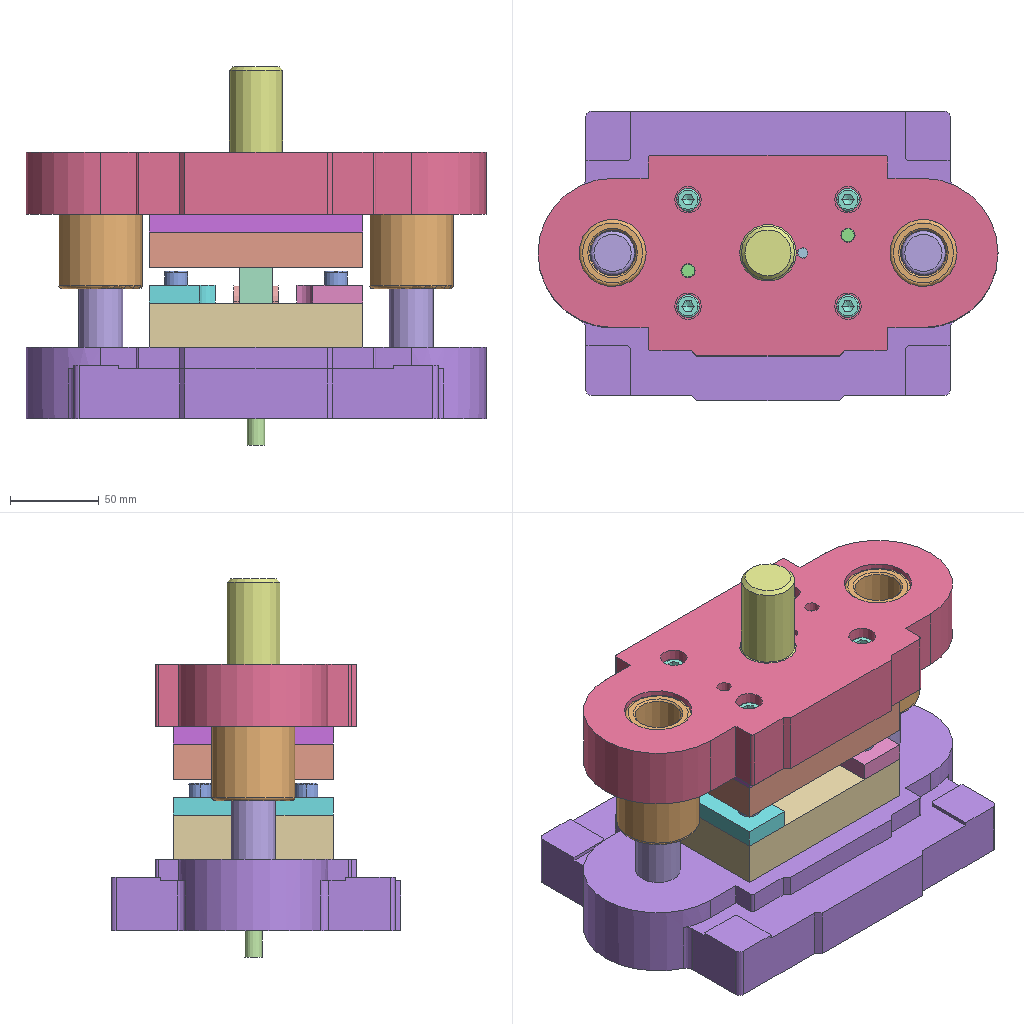Assembly | NX | 19 different items | 34 placed | box 259 x 163 x 213 mm
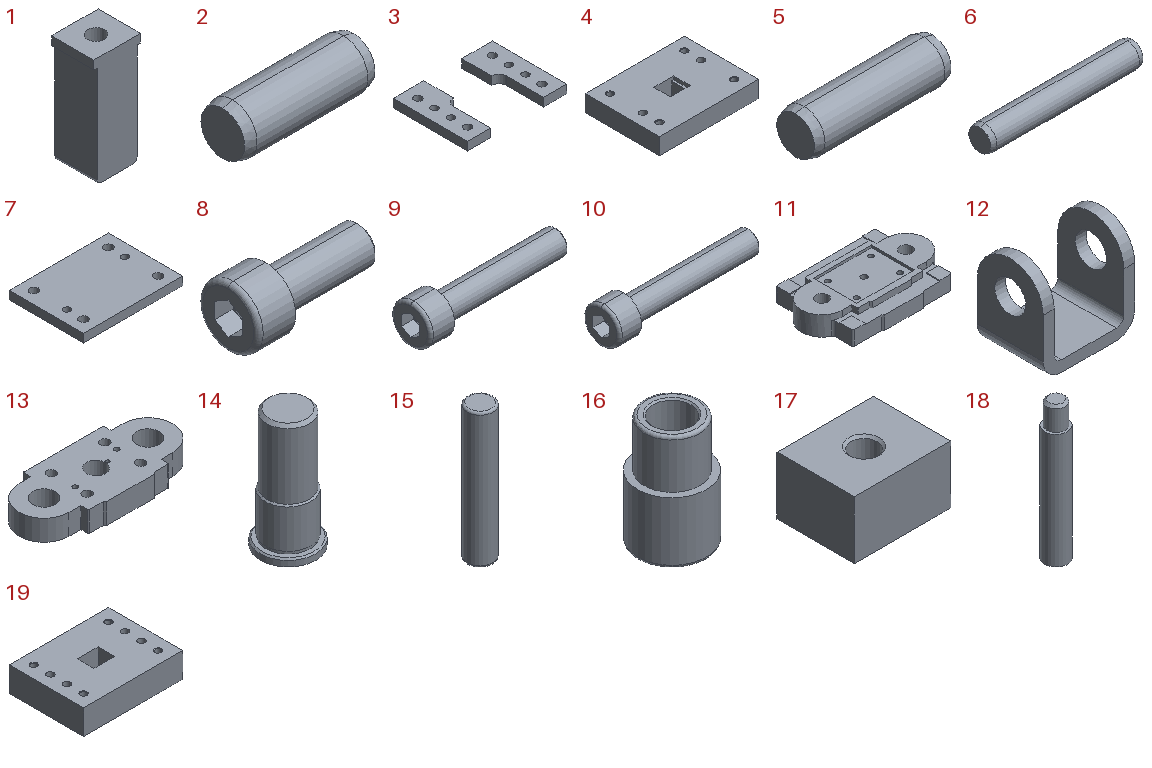Parts list (item | quantity | size | volume | features):
1 | x1 | 22 x 20 x 52 mm | 17352 mm3 | features EXTRUDE 3, DATUM_CSYS 2, BLEND 1, SKETCH 1
2 | x1 | 16 x 6 x 6 mm | 445.376 mm3 | features BREP 1
3 | x1 | 120 x 90 x 10 mm | 52672 mm3 | features DATUM_CSYS 1, EXTRUDE 1
4 | x1 | 120 x 90 x 20 mm | 203051 mm3 | features SIMPLE HOLE 4, SYMBOLIC_THREAD 4, EXTRUDE 2, DATUM_CSYS 1, HOLE PACKAGE 1
5 | x4 | 26 x 8 x 8 mm | 1290 mm3 | features BREP 1
6 | x2 | 50 x 8 x 8 mm | 2497 mm3 | features BREP 1
7 | x1 | 120 x 90 x 10 mm | 103853 mm3 | features DATUM_CSYS 1, EXTRUDE 1
8 | x4 | 28 x 13 x 13 mm | 1917 mm3 | features BREP 1
9 | x4 | 48 x 13 x 13 mm | 2922 mm3 | features BREP 1
10 | x4 | 53 x 13 x 13 mm | 3173 mm3 | features BREP 1
11 | x1 | 259 x 163 x 40 mm | 1193308 mm3 | features EXTRUDE 6, DATUM_CSYS 2, SKETCH 1
12 | x1 | 25 x 18 x 25 mm | 3015 mm3 | features DATUM_CSYS 6, EXTRUDE 5, SKETCH 5, EXTRACT_FACE 4, BLEND 2, Instance Feature 1, Mirror Feature 1
13 | x1 | 259 x 113 x 35 mm | 709332 mm3 | features EXTRUDE 3, DATUM_CSYS 2, SKETCH 1
14 | x1 | 38.769 x 39 x 83 mm | 63576 mm3 | features DATUM_CSYS 6, EXTRUDE 5, SKETCH 5, CHAMFER 2
15 | x2 | 25 x 25 x 130 mm | 63684 mm3 | features DATUM_CSYS 2, BLEND 1, EXTRUDE 1, SKETCH 1
16 | x2 | 47 x 47 x 75 mm | 71750 mm3 | features DATUM_CSYS 5, EXTRUDE 4, SKETCH 4, CHAMFER 2, BLEND 1
17 | x1 | 25 x 20 x 15 mm | 6947 mm3 | features DATUM_CSYS 1, EXTRUDE 1, HOLE PACKAGE 1, SIMPLE HOLE 1, SYMBOLIC_THREAD 1
18 | x1 | 10 x 10 x 60 mm | 4418 mm3 | features DATUM_CSYS 3, EXTRUDE 2, SKETCH 2, CHAMFER 1
19 | x1 | 120 x 90 x 30 mm | 298578 mm3 | features SIMPLE HOLE 4, SYMBOLIC_THREAD 4, DATUM_CSYS 1, EXTRUDE 1, HOLE PACKAGE 1
Mates (type | each side: item.copy, entity, surface, feature):
Touch | 19.1 face plane Extrude(1) | 11.1 face plane Extrude(6)
Touch | 15.1 face cylinder Extrude(1) | 11.1 face cylinder Extrude(1)
Touch | 9.1 face plane Body(1) | 11.1 face plane Extrude(5)
Touch | 9.1 face cylinder Body(1) | 11.1 face cylinder Extrude(4)
Touch | 3.1 face plane Extrude(1) | 19.1 face plane Extrude(1)
Touch | 18.1 face plane Extrude(1) | 11.1 face plane Extrude(6)
Touch | 17.1 face plane Extrude(1) | 11.1 face plane Extrude(6)
Touch | 8.1 face plane Body(1) | 3.1 face plane Extrude(1)
Touch | 8.1 face cylinder Body(1) | 3.1 face cylinder Extrude(1)
Touch | 5.1 face plane Body(1) | 3.1 face plane Extrude(1)
Touch | 5.1 face cylinder Body(1) | 3.1 face cylinder Extrude(1)
Distance | 4.1 face plane Extrude(1) | 3.1 face plane Extrude(1)
Distance | 1.1 face plane Extrude(1) | 4.1 face plane Extrude(1)
Touch | 7.1 face plane Extrude(1) | 4.1 face plane Extrude(1)
Touch | 14.1 face plane Extrude(1) | 7.1 face plane Extrude(1)
Touch | 2.1 face plane Body(1) | 7.1 face plane Extrude(1)
Touch | 2.1 face cylinder Body(1) | 14.1 face cylinder Extrude(7)
Touch | 13.1 face plane Extrude(1) | 7.1 face plane Extrude(1)
Touch | 16.1 face plane Extrude(1) | 13.1 face plane Extrude(1)
Touch | 16.1 face cylinder Extrude(2) | 13.1 face cylinder Extrude(1)
Touch | 10.1 face plane Body(1) | 13.1 face plane Extrude(2)
Touch | 10.1 face cylinder Body(1) | 13.1 face cylinder Extrude(2)
Distance | 6.1 face plane Body(1) | 13.1 face plane Extrude(1) | 2 times
Touch | 6.1 face cylinder Body(1) | 13.1 face cylinder Extrude(1) | 2 times
Touch | 12.1 face plane Extrude(1) | 17.1 face plane Extrude(1)